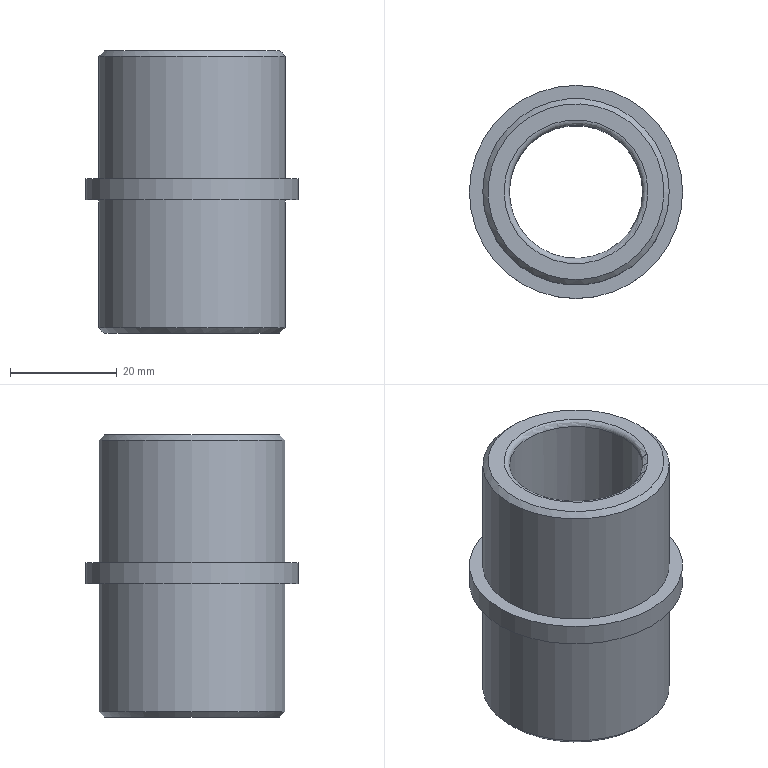Part | STEP file | solid 27 | 1 solid | 12 faces | box 40 x 40 x 53 mm | volume 26012 mm3 | plane 4 | cylinder 4 | cone 2 | torus 2 | commonest cylinder face diameters 35 x2 25 x1 40 x1